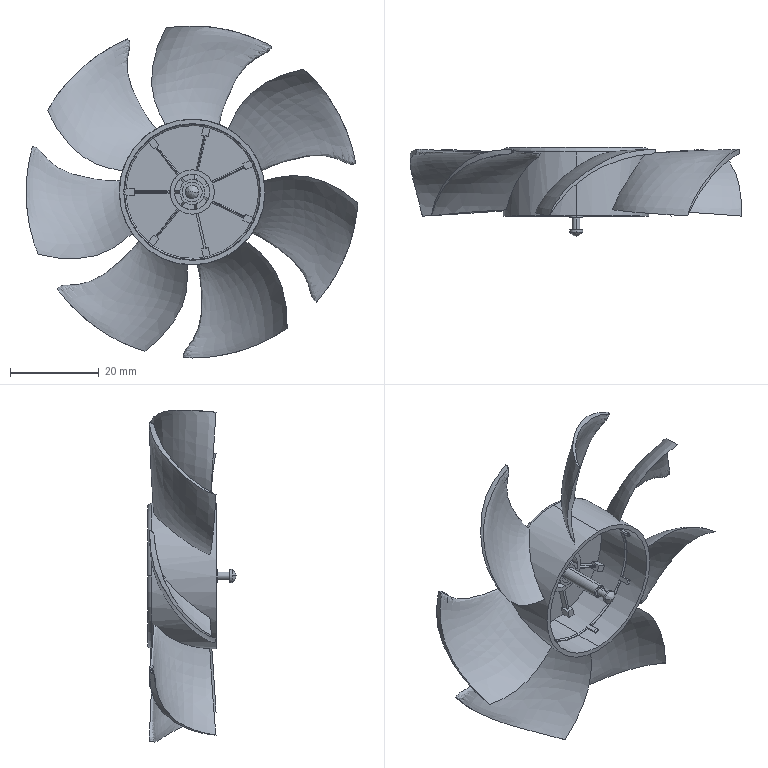Part | STEP file | 8025RYE_3_1.stp | 1 solid | 194 faces | box 74.924 x 20.1 x 75 mm | volume 5427 mm3 | plane 105 | cylinder 47 | torus 19 | spline 16 | cone 7 | commonest cylinder face diameters 0.4 x12 75 x8 26.1 x7 2.992 x4 1.8 x2 4.5 x2